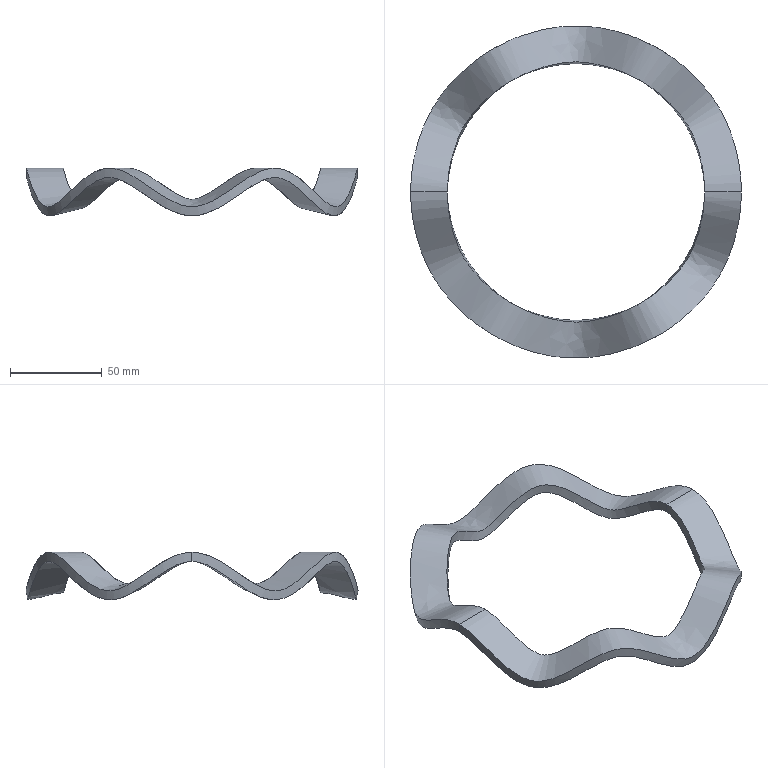Part | SolidWorks | features 3DProfileFeature 2, 3DSplineCurve 1, Extrusion 1, Sweep 1 | 1 solid | 8 faces | box 180 x 180.809 x 25.967 mm | volume 56026 mm3 | spline 8